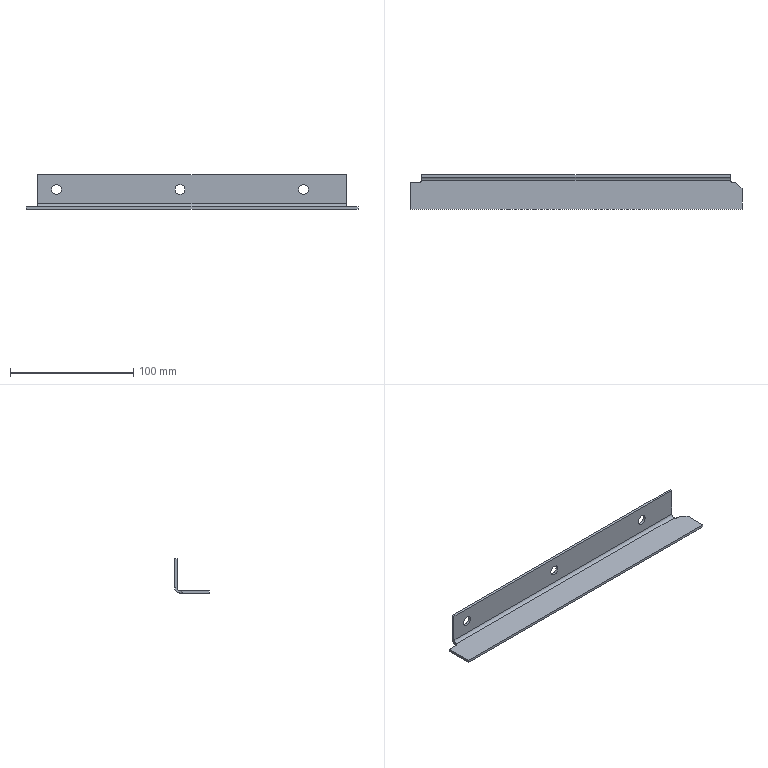Part | SolidWorks | features ICE 2, Chamfer 1, Fillet 1, FlatPattern 1, SMBaseFlange 1, SheetMetal 1 | 1 solid | 25 faces | box 268.9 x 28 x 28 mm | volume 26727 mm3 | plane 15 | cylinder 10 | commonest cylinder face diameters 8 x6 4 x2 5 x1 9 x1
STEP:
#1=CARTESIAN_POINT('',(-109.75,-2.,-16.));
#2=VERTEX_POINT('',#1);
#3=CARTESIAN_POINT('',(-109.75,-2.,-8.));
#4=VERTEX_POINT('',#3);
#5=CARTESIAN_POINT('',(-109.75,-2.,-12.));
#6=DIRECTION('',(0.,1.,0.));
#7=DIRECTION('',(0.,0.,1.));
#8=AXIS2_PLACEMENT_3D('',#5,#6,#7);
#9=CIRCLE('',#8,4.);
#10=EDGE_CURVE('',#2,#4,#9,.T.);
#11=ORIENTED_EDGE('',*,*,#10,.F.);
#12=CARTESIAN_POINT('',(-109.75,0.,-16.));
#13=VERTEX_POINT('',#12);
#14=CARTESIAN_POINT('',(-109.75,-28.,-16.));
#15=DIRECTION('',(0.,1.,0.));
#16=VECTOR('',#15,1000.);
#17=LINE('',#14,#16);
#18=EDGE_CURVE('',#2,#13,#17,.T.);
#19=ORIENTED_EDGE('',*,*,#18,.T.);
#20=CARTESIAN_POINT('',(-109.75,0.,-8.));
#21=VERTEX_POINT('',#20);
#22=CARTESIAN_POINT('',(-109.75,0.,-12.));
#23=DIRECTION('',(0.,1.,0.));
#24=DIRECTION('',(0.,0.,1.));
#25=AXIS2_PLACEMENT_3D('',#22,#23,#24);
#26=CIRCLE('',#25,4.);
#27=EDGE_CURVE('',#13,#21,#26,.T.);
#28=ORIENTED_EDGE('',*,*,#27,.T.);
#29=CARTESIAN_POINT('',(-109.75,-28.,-8.));
#30=DIRECTION('',(0.,1.,0.));
#31=VECTOR('',#30,1000.);
#32=LINE('',#29,#31);
#33=EDGE_CURVE('',#4,#21,#32,.T.);
#34=ORIENTED_EDGE('',*,*,#33,.F.);
#35=EDGE_LOOP('',(#11,#19,#28,#34));
#36=FACE_OUTER_BOUND('',#35,.T.);
#37=CARTESIAN_POINT('',(-109.75,-28.,-12.));
#38=DIRECTION('',(0.,1.,0.));
#39=DIRECTION('',(0.,0.,1.));
#40=AXIS2_PLACEMENT_3D('',#37,#38,#39);
#41=CYLINDRICAL_SURFACE('',#40,4.);
#42=ADVANCED_FACE('',(#36),#41,.F.);
#43=CARTESIAN_POINT('',(-9.75,-2.,-16.));
#44=VERTEX_POINT('',#43);
#45=CARTESIAN_POINT('',(-9.75,-2.,-8.));
#46=VERTEX_POINT('',#45);
#47=CARTESIAN_POINT('',(-9.75,-2.,-12.));
#48=DIRECTION('',(0.,1.,0.));
#49=DIRECTION('',(0.,0.,1.));
#50=AXIS2_PLACEMENT_3D('',#47,#48,#49);
#51=CIRCLE('',#50,4.);
#52=EDGE_CURVE('',#44,#46,#51,.T.);
#53=ORIENTED_EDGE('',*,*,#52,.F.);
#54=CARTESIAN_POINT('',(-9.75,0.,-16.));
#55=VERTEX_POINT('',#54);
#56=CARTESIAN_POINT('',(-9.75,-28.,-16.));
#57=DIRECTION('',(0.,1.,0.));
#58=VECTOR('',#57,1000.);
#59=LINE('',#56,#58);
#60=EDGE_CURVE('',#44,#55,#59,.T.);
#61=ORIENTED_EDGE('',*,*,#60,.T.);
#62=CARTESIAN_POINT('',(-9.75,0.,-8.));
#63=VERTEX_POINT('',#62);
#64=CARTESIAN_POINT('',(-9.75,0.,-12.));
#65=DIRECTION('',(0.,1.,0.));
#66=DIRECTION('',(0.,0.,1.));
#67=AXIS2_PLACEMENT_3D('',#64,#65,#66);
#68=CIRCLE('',#67,4.);
#69=EDGE_CURVE('',#55,#63,#68,.T.);
#70=ORIENTED_EDGE('',*,*,#69,.T.);
#71=CARTESIAN_POINT('',(-9.75,-28.,-8.));
#72=DIRECTION('',(0.,1.,0.));
#73=VECTOR('',#72,1000.);
#74=LINE('',#71,#73);
#75=EDGE_CURVE('',#46,#63,#74,.T.);
#76=ORIENTED_EDGE('',*,*,#75,.F.);
#77=EDGE_LOOP('',(#53,#61,#70,#76));
#78=FACE_OUTER_BOUND('',#77,.T.);
#79=CARTESIAN_POINT('',(-9.75,-28.,-12.));
#80=DIRECTION('',(0.,1.,0.));
#81=DIRECTION('',(0.,0.,1.));
#82=AXIS2_PLACEMENT_3D('',#79,#80,#81);
#83=CYLINDRICAL_SURFACE('',#82,4.);
#84=ADVANCED_FACE('',(#78),#83,.F.);
#85=CARTESIAN_POINT('',(90.25,-2.,-16.));
#86=VERTEX_POINT('',#85);
#87=CARTESIAN_POINT('',(90.25,-2.,-8.));
#88=VERTEX_POINT('',#87);
#89=CARTESIAN_POINT('',(90.25,-2.,-12.));
#90=DIRECTION('',(0.,1.,0.));
#91=DIRECTION('',(0.,0.,1.));
#92=AXIS2_PLACEMENT_3D('',#89,#90,#91);
#93=CIRCLE('',#92,4.);
#94=EDGE_CURVE('',#86,#88,#93,.T.);
#95=ORIENTED_EDGE('',*,*,#94,.F.);
#96=CARTESIAN_POINT('',(90.25,0.,-16.));
#97=VERTEX_POINT('',#96);
#98=CARTESIAN_POINT('',(90.25,-28.,-16.));
#99=DIRECTION('',(0.,1.,0.));
#100=VECTOR('',#99,1000.);
#101=LINE('',#98,#100);
#102=EDGE_CURVE('',#86,#97,#101,.T.);
#103=ORIENTED_EDGE('',*,*,#102,.T.);
#104=CARTESIAN_POINT('',(90.25,0.,-8.));
#105=VERTEX_POINT('',#104);
#106=CARTESIAN_POINT('',(90.25,0.,-12.));
#107=DIRECTION('',(0.,1.,0.));
#108=DIRECTION('',(0.,0.,1.));
#109=AXIS2_PLACEMENT_3D('',#106,#107,#108);
#110=CIRCLE('',#109,4.);
#111=EDGE_CURVE('',#97,#105,#110,.T.);
#112=ORIENTED_EDGE('',*,*,#111,.T.);
#113=CARTESIAN_POINT('',(90.25,-28.,-8.));
#114=DIRECTION('',(0.,1.,0.));
#115=VECTOR('',#114,1000.);
#116=LINE('',#113,#115);
#117=EDGE_CURVE('',#88,#105,#116,.T.);
#118=ORIENTED_EDGE('',*,*,#117,.F.);
#119=EDGE_LOOP('',(#95,#103,#112,#118));
#120=FACE_OUTER_BOUND('',#119,.T.);
#121=CARTESIAN_POINT('',(90.25,-28.,-12.));
#122=DIRECTION('',(0.,1.,0.));
#123=DIRECTION('',(0.,0.,1.));
#124=AXIS2_PLACEMENT_3D('',#121,#122,#123);
#125=CYLINDRICAL_SURFACE('',#124,4.);
#126=ADVANCED_FACE('',(#120),#125,.F.);
#127=CARTESIAN_POINT('',(124.75,-2.,-23.5));
#128=VERTEX_POINT('',#127);
#129=CARTESIAN_POINT('',(124.75,-2.,0.));
#130=VERTEX_POINT('',#129);
#131=CARTESIAN_POINT('',(124.75,-2.,0.));
#132=DIRECTION('',(0.,0.,1.));
#133=VECTOR('',#132,1000.);
#134=LINE('',#131,#133);
#135=EDGE_CURVE('',#128,#130,#134,.T.);
#136=ORIENTED_EDGE('',*,*,#135,.F.);
#137=CARTESIAN_POINT('',(124.75,0.,-23.5));
#138=VERTEX_POINT('',#137);
#139=CARTESIAN_POINT('',(124.75,-2.,-23.5));
#140=DIRECTION('',(0.,1.,0.));
#141=VECTOR('',#140,1000.);
#142=LINE('',#139,#141);
#143=EDGE_CURVE('',#128,#138,#142,.T.);
#144=ORIENTED_EDGE('',*,*,#143,.T.);
#145=CARTESIAN_POINT('',(124.75,0.,0.));
#146=VERTEX_POINT('',#145);
#147=CARTESIAN_POINT('',(124.75,0.,0.));
#148=DIRECTION('',(0.,0.,-1.));
#149=VECTOR('',#148,1000.);
#150=LINE('',#147,#149);
#151=EDGE_CURVE('',#146,#138,#150,.T.);
#152=ORIENTED_EDGE('',*,*,#151,.F.);
#153=CARTESIAN_POINT('',(124.75,0.,0.));
#154=DIRECTION('',(0.,1.,0.));
#155=VECTOR('',#154,1000.);
#156=LINE('',#153,#155);
#157=EDGE_CURVE('',#130,#146,#156,.T.);
#158=ORIENTED_EDGE('',*,*,#157,.F.);
#159=EDGE_LOOP('',(#136,#144,#152,#158));
#160=FACE_OUTER_BOUND('',#159,.T.);
#161=CARTESIAN_POINT('',(124.75,0.,0.));
#162=DIRECTION('',(-1.,0.,0.));
#163=DIRECTION('',(0.,0.,1.));
#164=AXIS2_PLACEMENT_3D('',#161,#162,#163);
#165=PLANE('',#164);
#166=ADVANCED_FACE('',(#160),#165,.F.);
#167=CARTESIAN_POINT('',(-124.75,0.,0.));
#168=VERTEX_POINT('',#167);
#169=CARTESIAN_POINT('',(-124.75,0.,-23.5));
#170=VERTEX_POINT('',#169);
#171=CARTESIAN_POINT('',(-124.75,0.,0.));
#172=DIRECTION('',(0.,0.,-1.));
#173=VECTOR('',#172,1000.);
#174=LINE('',#171,#173);
#175=EDGE_CURVE('',#168,#170,#174,.T.);
#176=ORIENTED_EDGE('',*,*,#175,.T.);
#177=CARTESIAN_POINT('',(-124.75,-2.,-23.5));
#178=VERTEX_POINT('',#177);
#179=CARTESIAN_POINT('',(-124.75,0.,-23.5));
#180=DIRECTION('',(0.,-1.,0.));
#181=VECTOR('',#180,1000.);
#182=LINE('',#179,#181);
#183=EDGE_CURVE('',#170,#178,#182,.T.);
#184=ORIENTED_EDGE('',*,*,#183,.T.);
#185=CARTESIAN_POINT('',(-124.75,-2.,0.));
#186=VERTEX_POINT('',#185);
#187=CARTESIAN_POINT('',(-124.75,-2.,0.));
#188=DIRECTION('',(0.,0.,-1.));
#189=VECTOR('',#188,1000.);
#190=LINE('',#187,#189);
#191=EDGE_CURVE('',#186,#178,#190,.T.);
#192=ORIENTED_EDGE('',*,*,#191,.F.);
#193=CARTESIAN_POINT('',(-124.75,0.,0.));
#194=DIRECTION('',(0.,-1.,0.));
#195=VECTOR('',#194,1000.);
#196=LINE('',#193,#195);
#197=EDGE_CURVE('',#168,#186,#196,.T.);
#198=ORIENTED_EDGE('',*,*,#197,.F.);
#199=EDGE_LOOP('',(#176,#184,#192,#198));
#200=FACE_OUTER_BOUND('',#199,.T.);
#201=CARTESIAN_POINT('',(-124.75,0.,0.));
#202=DIRECTION('',(1.,0.,0.));
#203=DIRECTION('',(0.,0.,-1.));
#204=AXIS2_PLACEMENT_3D('',#201,#202,#203);
#205=PLANE('',#204);
#206=ADVANCED_FACE('',(#200),#205,.F.);
#207=CARTESIAN_POINT('',(134.45,-11.,-28.));
#208=VERTEX_POINT('',#207);
#209=CARTESIAN_POINT('',(134.45,-28.,-28.));
#210=VERTEX_POINT('',#209);
#211=CARTESIAN_POINT('',(134.45,0.,-28.));
#212=DIRECTION('',(0.,-1.,0.));
#213=VECTOR('',#212,1000.);
#214=LINE('',#211,#213);
#215=EDGE_CURVE('',#208,#210,#214,.T.);
#216=ORIENTED_EDGE('',*,*,#215,.F.);
#217=CARTESIAN_POINT('',(134.45,-11.,-26.));
#218=VERTEX_POINT('',#217);
#219=CARTESIAN_POINT('',(134.45,-11.,-26.));
#220=DIRECTION('',(0.,0.,1.));
#221=VECTOR('',#220,1000.);
#222=LINE('',#219,#221);
#223=EDGE_CURVE('',#208,#218,#222,.T.);
#224=ORIENTED_EDGE('',*,*,#223,.T.);
#225=CARTESIAN_POINT('',(134.45,-28.,-26.));
#226=VERTEX_POINT('',#225);
#227=CARTESIAN_POINT('',(134.45,0.,-26.));
#228=DIRECTION('',(0.,-1.,0.));
#229=VECTOR('',#228,1000.);
#230=LINE('',#227,#229);
#231=EDGE_CURVE('',#218,#226,#230,.T.);
#232=ORIENTED_EDGE('',*,*,#231,.T.);
#233=CARTESIAN_POINT('',(134.45,-28.,-28.));
#234=DIRECTION('',(0.,0.,1.));
#235=VECTOR('',#234,1000.);
#236=LINE('',#233,#235);
#237=EDGE_CURVE('',#210,#226,#236,.T.);
#238=ORIENTED_EDGE('',*,*,#237,.F.);
#239=EDGE_LOOP('',(#216,#224,#232,#238));
#240=FACE_OUTER_BOUND('',#239,.T.);
#241=CARTESIAN_POINT('',(134.45,-2.,-23.5));
#242=DIRECTION('',(1.,0.,0.));
#243=DIRECTION('',(0.,0.,-1.));
#244=AXIS2_PLACEMENT_3D('',#241,#242,#243);
#245=PLANE('',#244);
#246=ADVANCED_FACE('',(#240),#245,.T.);
#247=ORIENTED_EDGE('',*,*,#231,.F.);
#248=CARTESIAN_POINT('',(129.45,-6.,-26.));
#249=VERTEX_POINT('',#248);
#250=CARTESIAN_POINT('',(129.45,-6.,-26.));
#251=DIRECTION('',(-0.7071,0.7071,0.));
#252=VECTOR('',#251,1000.);
#253=LINE('',#250,#252);
#254=EDGE_CURVE('',#218,#249,#253,.T.);
#255=ORIENTED_EDGE('',*,*,#254,.T.);
#256=CARTESIAN_POINT('',(126.75,-6.,-26.));
#257=VERTEX_POINT('',#256);
#258=CARTESIAN_POINT('',(134.45,-6.,-26.));
#259=DIRECTION('',(-1.,0.,0.));
#260=VECTOR('',#259,1000.);
#261=LINE('',#258,#260);
#262=EDGE_CURVE('',#249,#257,#261,.T.);
#263=ORIENTED_EDGE('',*,*,#262,.T.);
#264=CARTESIAN_POINT('',(124.814,-4.5,-26.));
#265=VERTEX_POINT('',#264);
#266=CARTESIAN_POINT('',(126.75,-4.,-26.));
#267=DIRECTION('',(0.,0.,-1.));
#268=DIRECTION('',(-1.,0.,0.));
#269=AXIS2_PLACEMENT_3D('',#266,#267,#268);
#270=CIRCLE('',#269,2.);
#271=EDGE_CURVE('',#257,#265,#270,.T.);
#272=ORIENTED_EDGE('',*,*,#271,.T.);
#273=CARTESIAN_POINT('',(-124.814,-4.5,-26.));
#274=VERTEX_POINT('',#273);
#275=CARTESIAN_POINT('',(134.45,-4.5,-26.));
#276=DIRECTION('',(-1.,0.,0.));
#277=VECTOR('',#276,1000.);
#278=LINE('',#275,#277);
#279=EDGE_CURVE('',#265,#274,#278,.T.);
#280=ORIENTED_EDGE('',*,*,#279,.T.);
#281=CARTESIAN_POINT('',(-126.75,-6.,-26.));
#282=VERTEX_POINT('',#281);
#283=CARTESIAN_POINT('',(-126.75,-4.,-26.));
#284=DIRECTION('',(0.,0.,-1.));
#285=DIRECTION('',(-1.,0.,0.));
#286=AXIS2_PLACEMENT_3D('',#283,#284,#285);
#287=CIRCLE('',#286,2.);
#288=EDGE_CURVE('',#274,#282,#287,.T.);
#289=ORIENTED_EDGE('',*,*,#288,.T.);
#290=CARTESIAN_POINT('',(-134.45,-6.,-26.));
#291=VERTEX_POINT('',#290);
#292=CARTESIAN_POINT('',(134.45,-6.,-26.));
#293=DIRECTION('',(-1.,0.,0.));
#294=VECTOR('',#293,1000.);
#295=LINE('',#292,#294);
#296=EDGE_CURVE('',#282,#291,#295,.T.);
#297=ORIENTED_EDGE('',*,*,#296,.T.);
#298=CARTESIAN_POINT('',(-134.45,-28.,-26.));
#299=VERTEX_POINT('',#298);
#300=CARTESIAN_POINT('',(-134.45,0.,-26.));
#301=DIRECTION('',(0.,-1.,0.));
#302=VECTOR('',#301,1000.);
#303=LINE('',#300,#302);
#304=EDGE_CURVE('',#291,#299,#303,.T.);
#305=ORIENTED_EDGE('',*,*,#304,.T.);
#306=CARTESIAN_POINT('',(134.45,-28.,-26.));
#307=DIRECTION('',(-1.,0.,0.));
#308=VECTOR('',#307,1000.);
#309=LINE('',#306,#308);
#310=EDGE_CURVE('',#226,#299,#309,.T.);
#311=ORIENTED_EDGE('',*,*,#310,.F.);
#312=EDGE_LOOP('',(#247,#255,#263,#272,#280,#289,#297,#305,#311));
#313=FACE_OUTER_BOUND('',#312,.T.);
#314=CARTESIAN_POINT('',(134.45,0.,-26.));
#315=DIRECTION('',(0.,0.,-1.));
#316=DIRECTION('',(-1.,0.,0.));
#317=AXIS2_PLACEMENT_3D('',#314,#315,#316);
#318=PLANE('',#317);
#319=ADVANCED_FACE('',(#313),#318,.F.);
#320=CARTESIAN_POINT('',(-134.45,-28.,-28.));
#321=VERTEX_POINT('',#320);
#322=CARTESIAN_POINT('',(-134.45,-28.,-28.));
#323=DIRECTION('',(0.,0.,1.));
#324=VECTOR('',#323,1000.);
#325=LINE('',#322,#324);
#326=EDGE_CURVE('',#321,#299,#325,.T.);
#327=ORIENTED_EDGE('',*,*,#326,.F.);
#328=CARTESIAN_POINT('',(134.45,-28.,-28.));
#329=DIRECTION('',(-1.,0.,0.));
#330=VECTOR('',#329,1000.);
#331=LINE('',#328,#330);
#332=EDGE_CURVE('',#210,#321,#331,.T.);
#333=ORIENTED_EDGE('',*,*,#332,.F.);
#334=ORIENTED_EDGE('',*,*,#237,.T.);
#335=ORIENTED_EDGE('',*,*,#310,.T.);
#336=EDGE_LOOP('',(#327,#333,#334,#335));
#337=FACE_OUTER_BOUND('',#336,.T.);
#338=CARTESIAN_POINT('',(134.45,-28.,-28.));
#339=DIRECTION('',(0.,-1.,0.));
#340=DIRECTION('',(0.,0.,-1.));
#341=AXIS2_PLACEMENT_3D('',#338,#339,#340);
#342=PLANE('',#341);
#343=ADVANCED_FACE('',(#337),#342,.T.);
#344=CARTESIAN_POINT('',(129.45,-6.,-28.));
#345=VERTEX_POINT('',#344);
#346=CARTESIAN_POINT('',(126.75,-6.,-28.));
#347=VERTEX_POINT('',#346);
#348=CARTESIAN_POINT('',(134.45,-6.,-28.));
#349=DIRECTION('',(-1.,0.,0.));
#350=VECTOR('',#349,1000.);
#351=LINE('',#348,#350);
#352=EDGE_CURVE('',#345,#347,#351,.T.);
#353=ORIENTED_EDGE('',*,*,#352,.F.);
#354=CARTESIAN_POINT('',(128.95,-5.5,-28.));
#355=DIRECTION('',(0.7071,-0.7071,0.));
#356=VECTOR('',#355,1000.);
#357=LINE('',#354,#356);
#358=EDGE_CURVE('',#345,#208,#357,.T.);
#359=ORIENTED_EDGE('',*,*,#358,.T.);
#360=ORIENTED_EDGE('',*,*,#215,.T.);
#361=ORIENTED_EDGE('',*,*,#332,.T.);
#362=CARTESIAN_POINT('',(-134.45,-6.,-28.));
#363=VERTEX_POINT('',#362);
#364=CARTESIAN_POINT('',(-134.45,0.,-28.));
#365=DIRECTION('',(0.,-1.,0.));
#366=VECTOR('',#365,1000.);
#367=LINE('',#364,#366);
#368=EDGE_CURVE('',#363,#321,#367,.T.);
#369=ORIENTED_EDGE('',*,*,#368,.F.);
#370=CARTESIAN_POINT('',(-126.75,-6.,-28.));
#371=VERTEX_POINT('',#370);
#372=CARTESIAN_POINT('',(-124.75,-6.,-28.));
#373=DIRECTION('',(-1.,0.,0.));
#374=VECTOR('',#373,1000.);
#375=LINE('',#372,#374);
#376=EDGE_CURVE('',#371,#363,#375,.T.);
#377=ORIENTED_EDGE('',*,*,#376,.F.);
#378=CARTESIAN_POINT('',(-124.814,-4.5,-28.));
#379=VERTEX_POINT('',#378);
#380=CARTESIAN_POINT('',(-126.75,-4.,-28.));
#381=DIRECTION('',(0.,0.,1.));
#382=DIRECTION('',(-1.,0.,0.));
#383=AXIS2_PLACEMENT_3D('',#380,#381,#382);
#384=CIRCLE('',#383,2.);
#385=EDGE_CURVE('',#371,#379,#384,.T.);
#386=ORIENTED_EDGE('',*,*,#385,.T.);
#387=CARTESIAN_POINT('',(124.814,-4.5,-28.));
#388=VERTEX_POINT('',#387);
#389=CARTESIAN_POINT('',(134.45,-4.5,-28.));
#390=DIRECTION('',(-1.,0.,0.));
#391=VECTOR('',#390,1000.);
#392=LINE('',#389,#391);
#393=EDGE_CURVE('',#388,#379,#392,.T.);
#394=ORIENTED_EDGE('',*,*,#393,.F.);
#395=CARTESIAN_POINT('',(126.75,-4.,-28.));
#396=DIRECTION('',(0.,0.,1.));
#397=DIRECTION('',(-1.,0.,0.));
#398=AXIS2_PLACEMENT_3D('',#395,#396,#397);
#399=CIRCLE('',#398,2.);
#400=EDGE_CURVE('',#388,#347,#399,.T.);
#401=ORIENTED_EDGE('',*,*,#400,.T.);
#402=EDGE_LOOP('',(#353,#359,#360,#361,#369,#377,#386,#394,#401));
#403=FACE_OUTER_BOUND('',#402,.T.);
#404=CARTESIAN_POINT('',(134.45,0.,-28.));
#405=DIRECTION('',(0.,0.,-1.));
#406=DIRECTION('',(-1.,0.,0.));
#407=AXIS2_PLACEMENT_3D('',#404,#405,#406);
#408=PLANE('',#407);
#409=ADVANCED_FACE('',(#403),#408,.T.);
#410=CARTESIAN_POINT('',(-124.75,-4.,-27.972));
#411=VERTEX_POINT('',#410);
#412=CARTESIAN_POINT('',(-124.75,-4.5,-23.5));
#413=DIRECTION('',(-1.,0.,0.));
#414=DIRECTION('',(0.,0.,-1.));
#415=AXIS2_PLACEMENT_3D('',#412,#413,#414);
#416=CIRCLE('',#415,4.5);
#417=EDGE_CURVE('',#170,#411,#416,.T.);
#418=ORIENTED_EDGE('',*,*,#417,.F.);
#419=CARTESIAN_POINT('',(134.45,0.,-23.5));
#420=DIRECTION('',(-1.,0.,0.));
#421=VECTOR('',#420,1000.);
#422=LINE('',#419,#421);
#423=EDGE_CURVE('',#138,#170,#422,.T.);
#424=ORIENTED_EDGE('',*,*,#423,.F.);
#425=CARTESIAN_POINT('',(124.75,-4.,-27.972));
#426=VERTEX_POINT('',#425);
#427=CARTESIAN_POINT('',(124.75,-4.5,-23.5));
#428=DIRECTION('',(1.,0.,0.));
#429=DIRECTION('',(0.,0.,1.));
#430=AXIS2_PLACEMENT_3D('',#427,#428,#429);
#431=CIRCLE('',#430,4.5);
#432=EDGE_CURVE('',#426,#138,#431,.T.);
#433=ORIENTED_EDGE('',*,*,#432,.F.);
#434=CARTESIAN_POINT('',(124.75,-4.,-27.972));
#435=CARTESIAN_POINT('',(124.75,-4.169,-27.991));
#436=CARTESIAN_POINT('',(124.771,-4.336,-28.));
#437=CARTESIAN_POINT('',(124.814,-4.5,-28.));
#438=B_SPLINE_CURVE_WITH_KNOTS('',3,(#434,#435,#436,#437),.UNSPECIFIED.,.F.,.F.,(4,4),(0.,0.0005048),.UNSPECIFIED.);
#439=EDGE_CURVE('',#426,#388,#438,.T.);
#440=ORIENTED_EDGE('',*,*,#439,.T.);
#441=ORIENTED_EDGE('',*,*,#393,.T.);
#442=CARTESIAN_POINT('',(-124.814,-4.5,-28.));
#443=CARTESIAN_POINT('',(-124.771,-4.336,-28.));
#444=CARTESIAN_POINT('',(-124.75,-4.169,-27.991));
#445=CARTESIAN_POINT('',(-124.75,-4.,-27.972));
#446=B_SPLINE_CURVE_WITH_KNOTS('',3,(#442,#443,#444,#445),.UNSPECIFIED.,.F.,.F.,(4,4),(0.,0.0005048),.UNSPECIFIED.);
#447=EDGE_CURVE('',#379,#411,#446,.T.);
#448=ORIENTED_EDGE('',*,*,#447,.T.);
#449=EDGE_LOOP('',(#418,#424,#433,#440,#441,#448));
#450=FACE_OUTER_BOUND('',#449,.T.);
#451=CARTESIAN_POINT('',(134.45,-4.5,-23.5));
#452=DIRECTION('',(-1.,0.,0.));
#453=DIRECTION('',(0.,0.,1.));
#454=AXIS2_PLACEMENT_3D('',#451,#452,#453);
#455=CYLINDRICAL_SURFACE('',#454,4.5);
#456=ADVANCED_FACE('',(#450),#455,.T.);
#457=CARTESIAN_POINT('',(-109.75,0.,-12.));
#458=DIRECTION('',(0.,1.,0.));
#459=DIRECTION('',(0.,0.,1.));
#460=AXIS2_PLACEMENT_3D('',#457,#458,#459);
#461=CIRCLE('',#460,4.);
#462=EDGE_CURVE('',#21,#13,#461,.T.);
#463=ORIENTED_EDGE('',*,*,#462,.F.);
#464=ORIENTED_EDGE('',*,*,#27,.F.);
#465=EDGE_LOOP('',(#463,#464));
#466=FACE_BOUND('',#465,.T.);
#467=CARTESIAN_POINT('',(-9.75,0.,-12.));
#468=DIRECTION('',(0.,1.,0.));
#469=DIRECTION('',(0.,0.,1.));
#470=AXIS2_PLACEMENT_3D('',#467,#468,#469);
#471=CIRCLE('',#470,4.);
#472=EDGE_CURVE('',#63,#55,#471,.T.);
#473=ORIENTED_EDGE('',*,*,#472,.F.);
#474=ORIENTED_EDGE('',*,*,#69,.F.);
#475=EDGE_LOOP('',(#473,#474));
#476=FACE_BOUND('',#475,.T.);
#477=CARTESIAN_POINT('',(90.25,0.,-12.));
#478=DIRECTION('',(0.,1.,0.));
#479=DIRECTION('',(0.,0.,1.));
#480=AXIS2_PLACEMENT_3D('',#477,#478,#479);
#481=CIRCLE('',#480,4.);
#482=EDGE_CURVE('',#105,#97,#481,.T.);
#483=ORIENTED_EDGE('',*,*,#482,.F.);
#484=ORIENTED_EDGE('',*,*,#111,.F.);
#485=EDGE_LOOP('',(#483,#484));
#486=FACE_BOUND('',#485,.T.);
#487=ORIENTED_EDGE('',*,*,#175,.F.);
#488=CARTESIAN_POINT('',(134.45,0.,0.));
#489=DIRECTION('',(-1.,0.,0.));
#490=VECTOR('',#489,1000.);
#491=LINE('',#488,#490);
#492=EDGE_CURVE('',#146,#168,#491,.T.);
#493=ORIENTED_EDGE('',*,*,#492,.F.);
#494=ORIENTED_EDGE('',*,*,#151,.T.);
#495=ORIENTED_EDGE('',*,*,#423,.T.);
#496=EDGE_LOOP('',(#487,#493,#494,#495));
#497=FACE_OUTER_BOUND('',#496,.T.);
#498=CARTESIAN_POINT('',(134.45,0.,0.));
#499=DIRECTION('',(0.,1.,0.));
#500=DIRECTION('',(0.,0.,1.));
#501=AXIS2_PLACEMENT_3D('',#498,#499,#500);
#502=PLANE('',#501);
#503=ADVANCED_FACE('',(#466,#476,#486,#497),#502,.T.);
#504=ORIENTED_EDGE('',*,*,#197,.T.);
#505=CARTESIAN_POINT('',(134.45,-2.,0.));
#506=DIRECTION('',(-1.,0.,0.));
#507=VECTOR('',#506,1000.);
#508=LINE('',#505,#507);
#509=EDGE_CURVE('',#130,#186,#508,.T.);
#510=ORIENTED_EDGE('',*,*,#509,.F.);
#511=ORIENTED_EDGE('',*,*,#157,.T.);
#512=ORIENTED_EDGE('',*,*,#492,.T.);
#513=EDGE_LOOP('',(#504,#510,#511,#512));
#514=FACE_OUTER_BOUND('',#513,.T.);
#515=CARTESIAN_POINT('',(134.45,-2.,0.));
#516=DIRECTION('',(0.,0.,1.));
#517=DIRECTION('',(1.,0.,0.));
#518=AXIS2_PLACEMENT_3D('',#515,#516,#517);
#519=PLANE('',#518);
#520=ADVANCED_FACE('',(#514),#519,.T.);
#521=CARTESIAN_POINT('',(-109.75,-2.,-12.));
#522=DIRECTION('',(0.,1.,0.));
#523=DIRECTION('',(0.,0.,1.));
#524=AXIS2_PLACEMENT_3D('',#521,#522,#523);
#525=CIRCLE('',#524,4.);
#526=EDGE_CURVE('',#4,#2,#525,.T.);
#527=ORIENTED_EDGE('',*,*,#526,.T.);
#528=ORIENTED_EDGE('',*,*,#10,.T.);
#529=EDGE_LOOP('',(#527,#528));
#530=FACE_BOUND('',#529,.T.);
#531=CARTESIAN_POINT('',(-9.75,-2.,-12.));
#532=DIRECTION('',(0.,1.,0.));
#533=DIRECTION('',(0.,0.,1.));
#534=AXIS2_PLACEMENT_3D('',#531,#532,#533);
#535=CIRCLE('',#534,4.);
#536=EDGE_CURVE('',#46,#44,#535,.T.);
#537=ORIENTED_EDGE('',*,*,#536,.T.);
#538=ORIENTED_EDGE('',*,*,#52,.T.);
#539=EDGE_LOOP('',(#537,#538));
#540=FACE_BOUND('',#539,.T.);
#541=CARTESIAN_POINT('',(90.25,-2.,-12.));
#542=DIRECTION('',(0.,1.,0.));
#543=DIRECTION('',(0.,0.,1.));
#544=AXIS2_PLACEMENT_3D('',#541,#542,#543);
#545=CIRCLE('',#544,4.);
#546=EDGE_CURVE('',#88,#86,#545,.T.);
#547=ORIENTED_EDGE('',*,*,#546,.T.);
#548=ORIENTED_EDGE('',*,*,#94,.T.);
#549=EDGE_LOOP('',(#547,#548));
#550=FACE_BOUND('',#549,.T.);
#551=ORIENTED_EDGE('',*,*,#509,.T.);
#552=ORIENTED_EDGE('',*,*,#191,.T.);
#553=CARTESIAN_POINT('',(134.45,-2.,-23.5));
#554=DIRECTION('',(-1.,0.,0.));
#555=VECTOR('',#554,1000.);
#556=LINE('',#553,#555);
#557=EDGE_CURVE('',#128,#178,#556,.T.);
#558=ORIENTED_EDGE('',*,*,#557,.F.);
#559=ORIENTED_EDGE('',*,*,#135,.T.);
#560=EDGE_LOOP('',(#551,#552,#558,#559));
#561=FACE_OUTER_BOUND('',#560,.T.);
#562=CARTESIAN_POINT('',(134.45,-2.,0.));
#563=DIRECTION('',(0.,1.,0.));
#564=DIRECTION('',(0.,0.,1.));
#565=AXIS2_PLACEMENT_3D('',#562,#563,#564);
#566=PLANE('',#565);
#567=ADVANCED_FACE('',(#530,#540,#550,#561),#566,.F.);
#568=ORIENTED_EDGE('',*,*,#557,.T.);
#569=CARTESIAN_POINT('',(-124.75,-4.,-25.949));
#570=VERTEX_POINT('',#569);
#571=CARTESIAN_POINT('',(-124.75,-4.5,-23.5));
#572=DIRECTION('',(-1.,0.,0.));
#573=DIRECTION('',(0.,0.,-1.));
#574=AXIS2_PLACEMENT_3D('',#571,#572,#573);
#575=CIRCLE('',#574,2.5);
#576=EDGE_CURVE('',#178,#570,#575,.T.);
#577=ORIENTED_EDGE('',*,*,#576,.T.);
#578=CARTESIAN_POINT('',(-124.75,-4.,-25.949));
#579=CARTESIAN_POINT('',(-124.75,-4.168,-25.984));
#580=CARTESIAN_POINT('',(-124.771,-4.334,-26.));
#581=CARTESIAN_POINT('',(-124.814,-4.5,-26.));
#582=B_SPLINE_CURVE_WITH_KNOTS('',3,(#578,#579,#580,#581),.UNSPECIFIED.,.F.,.F.,(4,4),(0.,0.0005065),.UNSPECIFIED.);
#583=EDGE_CURVE('',#570,#274,#582,.T.);
#584=ORIENTED_EDGE('',*,*,#583,.T.);
#585=ORIENTED_EDGE('',*,*,#279,.F.);
#586=CARTESIAN_POINT('',(124.75,-4.,-25.949));
#587=VERTEX_POINT('',#586);
#588=CARTESIAN_POINT('',(124.814,-4.5,-26.));
#589=CARTESIAN_POINT('',(124.771,-4.334,-26.));
#590=CARTESIAN_POINT('',(124.75,-4.168,-25.984));
#591=CARTESIAN_POINT('',(124.75,-4.,-25.949));
#592=B_SPLINE_CURVE_WITH_KNOTS('',3,(#588,#589,#590,#591),.UNSPECIFIED.,.F.,.F.,(4,4),(0.,0.0005065),.UNSPECIFIED.);
#593=EDGE_CURVE('',#265,#587,#592,.T.);
#594=ORIENTED_EDGE('',*,*,#593,.T.);
#595=CARTESIAN_POINT('',(124.75,-4.5,-23.5));
#596=DIRECTION('',(1.,0.,0.));
#597=DIRECTION('',(0.,0.,1.));
#598=AXIS2_PLACEMENT_3D('',#595,#596,#597);
#599=CIRCLE('',#598,2.5);
#600=EDGE_CURVE('',#587,#128,#599,.T.);
#601=ORIENTED_EDGE('',*,*,#600,.T.);
#602=EDGE_LOOP('',(#568,#577,#584,#585,#594,#601));
#603=FACE_OUTER_BOUND('',#602,.T.);
#604=CARTESIAN_POINT('',(134.45,-4.5,-23.5));
#605=DIRECTION('',(-1.,0.,0.));
#606=DIRECTION('',(0.,0.,1.));
#607=AXIS2_PLACEMENT_3D('',#604,#605,#606);
#608=CYLINDRICAL_SURFACE('',#607,2.5);
#609=ADVANCED_FACE('',(#603),#608,.F.);
#610=ORIENTED_EDGE('',*,*,#304,.F.);
#611=CARTESIAN_POINT('',(-134.45,-6.,-23.5));
#612=DIRECTION('',(0.,0.,-1.));
#613=VECTOR('',#612,1000.);
#614=LINE('',#611,#613);
#615=EDGE_CURVE('',#291,#363,#614,.T.);
#616=ORIENTED_EDGE('',*,*,#615,.T.);
#617=ORIENTED_EDGE('',*,*,#368,.T.);
#618=ORIENTED_EDGE('',*,*,#326,.T.);
#619=EDGE_LOOP('',(#610,#616,#617,#618));
#620=FACE_OUTER_BOUND('',#619,.T.);
#621=CARTESIAN_POINT('',(-134.45,-4.5,-23.5));
#622=DIRECTION('',(1.,0.,0.));
#623=DIRECTION('',(0.,0.,-1.));
#624=AXIS2_PLACEMENT_3D('',#621,#622,#623);
#625=PLANE('',#624);
#626=ADVANCED_FACE('',(#620),#625,.F.);
#627=ORIENTED_EDGE('',*,*,#417,.T.);
#628=CARTESIAN_POINT('',(-124.75,-4.,-26.));
#629=DIRECTION('',(0.,0.,1.));
#630=VECTOR('',#629,1000.);
#631=LINE('',#628,#630);
#632=EDGE_CURVE('',#411,#570,#631,.T.);
#633=ORIENTED_EDGE('',*,*,#632,.T.);
#634=ORIENTED_EDGE('',*,*,#576,.F.);
#635=ORIENTED_EDGE('',*,*,#183,.F.);
#636=EDGE_LOOP('',(#627,#633,#634,#635));
#637=FACE_OUTER_BOUND('',#636,.T.);
#638=CARTESIAN_POINT('',(-124.75,0.,0.));
#639=DIRECTION('',(1.,0.,0.));
#640=DIRECTION('',(0.,0.,-1.));
#641=AXIS2_PLACEMENT_3D('',#638,#639,#640);
#642=PLANE('',#641);
#643=ADVANCED_FACE('',(#637),#642,.F.);
#644=ORIENTED_EDGE('',*,*,#296,.F.);
#645=CARTESIAN_POINT('',(-126.75,-6.,-28.));
#646=DIRECTION('',(0.,0.,-1.));
#647=VECTOR('',#646,1000.);
#648=LINE('',#645,#647);
#649=EDGE_CURVE('',#282,#371,#648,.T.);
#650=ORIENTED_EDGE('',*,*,#649,.T.);
#651=ORIENTED_EDGE('',*,*,#376,.T.);
#652=ORIENTED_EDGE('',*,*,#615,.F.);
#653=EDGE_LOOP('',(#644,#650,#651,#652));
#654=FACE_OUTER_BOUND('',#653,.T.);
#655=CARTESIAN_POINT('',(-124.75,-6.,0.));
#656=DIRECTION('',(0.,-1.,0.));
#657=DIRECTION('',(0.,0.,-1.));
#658=AXIS2_PLACEMENT_3D('',#655,#656,#657);
#659=PLANE('',#658);
#660=ADVANCED_FACE('',(#654),#659,.F.);
#661=ORIENTED_EDGE('',*,*,#352,.T.);
#662=CARTESIAN_POINT('',(126.75,-6.,-26.));
#663=DIRECTION('',(0.,0.,1.));
#664=VECTOR('',#663,1000.);
#665=LINE('',#662,#664);
#666=EDGE_CURVE('',#347,#257,#665,.T.);
#667=ORIENTED_EDGE('',*,*,#666,.T.);
#668=ORIENTED_EDGE('',*,*,#262,.F.);
#669=CARTESIAN_POINT('',(129.45,-6.,-28.));
#670=DIRECTION('',(0.,0.,-1.));
#671=VECTOR('',#670,1000.);
#672=LINE('',#669,#671);
#673=EDGE_CURVE('',#249,#345,#672,.T.);
#674=ORIENTED_EDGE('',*,*,#673,.T.);
#675=EDGE_LOOP('',(#661,#667,#668,#674));
#676=FACE_OUTER_BOUND('',#675,.T.);
#677=CARTESIAN_POINT('',(134.45,-6.,0.));
#678=DIRECTION('',(0.,-1.,0.));
#679=DIRECTION('',(0.,0.,-1.));
#680=AXIS2_PLACEMENT_3D('',#677,#678,#679);
#681=PLANE('',#680);
#682=ADVANCED_FACE('',(#676),#681,.F.);
#683=ORIENTED_EDGE('',*,*,#600,.F.);
#684=CARTESIAN_POINT('',(124.75,-4.,-28.));
#685=DIRECTION('',(0.,0.,-1.));
#686=VECTOR('',#685,1000.);
#687=LINE('',#684,#686);
#688=EDGE_CURVE('',#587,#426,#687,.T.);
#689=ORIENTED_EDGE('',*,*,#688,.T.);
#690=ORIENTED_EDGE('',*,*,#432,.T.);
#691=ORIENTED_EDGE('',*,*,#143,.F.);
#692=EDGE_LOOP('',(#683,#689,#690,#691));
#693=FACE_OUTER_BOUND('',#692,.T.);
#694=CARTESIAN_POINT('',(124.75,0.,0.));
#695=DIRECTION('',(-1.,0.,0.));
#696=DIRECTION('',(0.,0.,1.));
#697=AXIS2_PLACEMENT_3D('',#694,#695,#696);
#698=PLANE('',#697);
#699=ADVANCED_FACE('',(#693),#698,.F.);
#700=ORIENTED_EDGE('',*,*,#102,.F.);
#701=ORIENTED_EDGE('',*,*,#546,.F.);
#702=ORIENTED_EDGE('',*,*,#117,.T.);
#703=ORIENTED_EDGE('',*,*,#482,.T.);
#704=EDGE_LOOP('',(#700,#701,#702,#703));
#705=FACE_OUTER_BOUND('',#704,.T.);
#706=CARTESIAN_POINT('',(90.25,-28.,-12.));
#707=DIRECTION('',(0.,1.,0.));
#708=DIRECTION('',(0.,0.,1.));
#709=AXIS2_PLACEMENT_3D('',#706,#707,#708);
#710=CYLINDRICAL_SURFACE('',#709,4.);
#711=ADVANCED_FACE('',(#705),#710,.F.);
#712=ORIENTED_EDGE('',*,*,#60,.F.);
#713=ORIENTED_EDGE('',*,*,#536,.F.);
#714=ORIENTED_EDGE('',*,*,#75,.T.);
#715=ORIENTED_EDGE('',*,*,#472,.T.);
#716=EDGE_LOOP('',(#712,#713,#714,#715));
#717=FACE_OUTER_BOUND('',#716,.T.);
#718=CARTESIAN_POINT('',(-9.75,-28.,-12.));
#719=DIRECTION('',(0.,1.,0.));
#720=DIRECTION('',(0.,0.,1.));
#721=AXIS2_PLACEMENT_3D('',#718,#719,#720);
#722=CYLINDRICAL_SURFACE('',#721,4.);
#723=ADVANCED_FACE('',(#717),#722,.F.);
#724=ORIENTED_EDGE('',*,*,#18,.F.);
#725=ORIENTED_EDGE('',*,*,#526,.F.);
#726=ORIENTED_EDGE('',*,*,#33,.T.);
#727=ORIENTED_EDGE('',*,*,#462,.T.);
#728=EDGE_LOOP('',(#724,#725,#726,#727));
#729=FACE_OUTER_BOUND('',#728,.T.);
#730=CARTESIAN_POINT('',(-109.75,-28.,-12.));
#731=DIRECTION('',(0.,1.,0.));
#732=DIRECTION('',(0.,0.,1.));
#733=AXIS2_PLACEMENT_3D('',#730,#731,#732);
#734=CYLINDRICAL_SURFACE('',#733,4.);
#735=ADVANCED_FACE('',(#729),#734,.F.);
#736=ORIENTED_EDGE('',*,*,#254,.F.);
#737=ORIENTED_EDGE('',*,*,#223,.F.);
#738=ORIENTED_EDGE('',*,*,#358,.F.);
#739=ORIENTED_EDGE('',*,*,#673,.F.);
#740=EDGE_LOOP('',(#736,#737,#738,#739));
#741=FACE_OUTER_BOUND('',#740,.T.);
#742=CARTESIAN_POINT('',(129.45,-6.,0.));
#743=DIRECTION('',(0.7071,0.7071,0.));
#744=DIRECTION('',(0.,0.,1.));
#745=AXIS2_PLACEMENT_3D('',#742,#743,#744);
#746=PLANE('',#745);
#747=ADVANCED_FACE('',(#741),#746,.T.);
#748=ORIENTED_EDGE('',*,*,#583,.F.);
#749=ORIENTED_EDGE('',*,*,#632,.F.);
#750=ORIENTED_EDGE('',*,*,#447,.F.);
#751=ORIENTED_EDGE('',*,*,#385,.F.);
#752=ORIENTED_EDGE('',*,*,#649,.F.);
#753=ORIENTED_EDGE('',*,*,#288,.F.);
#754=EDGE_LOOP('',(#748,#749,#750,#751,#752,#753));
#755=FACE_OUTER_BOUND('',#754,.T.);
#756=CARTESIAN_POINT('',(-126.75,-4.,0.));
#757=DIRECTION('',(0.,0.,1.));
#758=DIRECTION('',(1.,0.,0.));
#759=AXIS2_PLACEMENT_3D('',#756,#757,#758);
#760=CYLINDRICAL_SURFACE('',#759,2.);
#761=ADVANCED_FACE('',(#755),#760,.F.);
#762=ORIENTED_EDGE('',*,*,#271,.F.);
#763=ORIENTED_EDGE('',*,*,#666,.F.);
#764=ORIENTED_EDGE('',*,*,#400,.F.);
#765=ORIENTED_EDGE('',*,*,#439,.F.);
#766=ORIENTED_EDGE('',*,*,#688,.F.);
#767=ORIENTED_EDGE('',*,*,#593,.F.);
#768=EDGE_LOOP('',(#762,#763,#764,#765,#766,#767));
#769=FACE_OUTER_BOUND('',#768,.T.);
#770=CARTESIAN_POINT('',(126.75,-4.,0.));
#771=DIRECTION('',(0.,0.,1.));
#772=DIRECTION('',(1.,0.,0.));
#773=AXIS2_PLACEMENT_3D('',#770,#771,#772);
#774=CYLINDRICAL_SURFACE('',#773,2.);
#775=ADVANCED_FACE('',(#769),#774,.F.);
#776=CLOSED_SHELL('',(#42,#84,#126,#166,#206,#246,#319,#343,#409,#456,#503,#520,#567,#609,#626,#643,#660,#682,#699,#711,#723,#735,#747,#761,#775));
#777=MANIFOLD_SOLID_BREP('',#776);
#778=CARTESIAN_POINT('',(0.,0.,0.));
#779=DIRECTION('',(0.,0.,1.));
#780=DIRECTION('',(1.,0.,0.));
#781=AXIS2_PLACEMENT_3D('',#778,#779,#780);
#782=(LENGTH_UNIT()NAMED_UNIT(*)SI_UNIT(.MILLI.,.METRE.));
#783=UNCERTAINTY_MEASURE_WITH_UNIT(LENGTH_MEASURE(0.00001),#782,'','');
#784=(NAMED_UNIT(*)PLANE_ANGLE_UNIT()SI_UNIT($,.RADIAN.));
#785=(NAMED_UNIT(*)SI_UNIT($,.STERADIAN.)SOLID_ANGLE_UNIT());
#786=(GEOMETRIC_REPRESENTATION_CONTEXT(3)GLOBAL_UNCERTAINTY_ASSIGNED_CONTEXT((#783))GLOBAL_UNIT_ASSIGNED_CONTEXT((#782,#784,#785))REPRESENTATION_CONTEXT('',''));
#787=ADVANCED_BREP_SHAPE_REPRESENTATION('',(#777,#781),#786);